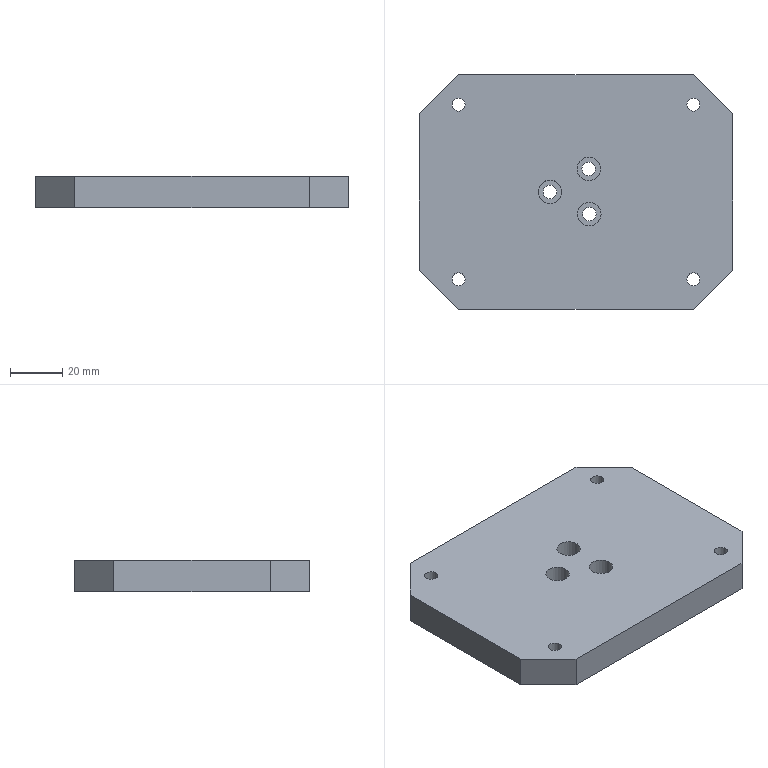Part | STEP file | 1 solid | 23 faces | box 120 x 90 x 12 mm | volume 121667 mm3 | plane 13 | cylinder 10 | commonest cylinder face diameters 5 x4 5.2 x3 9 x3